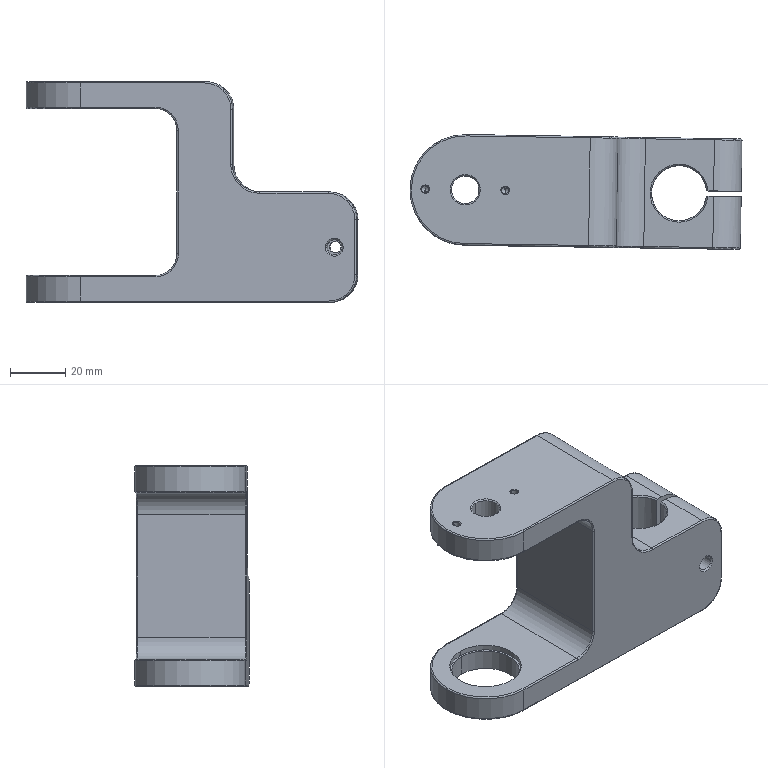Part | SolidWorks | features BaseBody 1 | 1 solid | 129 faces | box 120.282 x 41.496 x 80 mm | volume 152612 mm3 | cylinder 50 | spline 32 | cone 27 | plane 20 | commonest cylinder face diameters 1 x17 20 x9 2.5 x4 2.65 x4 40 x4 4.2 x2